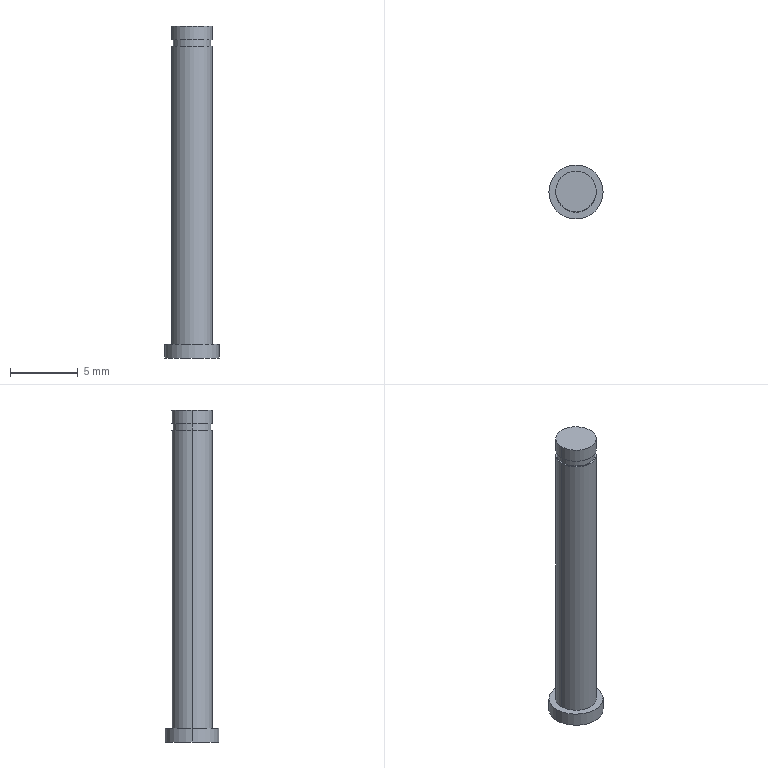Part | STEP file | PN_0099 pin shaft | 1 solid | 13 faces | box 4 x 4 x 24.5 mm | volume 178.223 mm3 | cylinder 8 | plane 5 | commonest cylinder face diameters 3 x4 2.8 x2 4 x2
STEP:
#1=CARTESIAN_POINT('',(0.,0.,0.));
#2=DIRECTION('',(0.,0.,1.));
#3=DIRECTION('',(1.,0.,0.));
#4=AXIS2_PLACEMENT_3D('',#1,#2,#3);
#5=CARTESIAN_POINT('',(1.5,0.,23.5));
#6=VERTEX_POINT('',#5);
#7=CARTESIAN_POINT('',(-1.5,0.,23.5));
#8=VERTEX_POINT('',#7);
#9=CARTESIAN_POINT('',(0.,0.,23.5));
#10=DIRECTION('',(0.,0.,1.));
#11=DIRECTION('',(1.,0.,0.));
#12=AXIS2_PLACEMENT_3D('',#9,#10,#11);
#13=CIRCLE('',#12,1.5);
#14=CARTESIAN_POINT('',(0.,0.,23.5));
#15=DIRECTION('',(0.,0.,-1.));
#16=DIRECTION('',(-1.,0.,0.));
#17=AXIS2_PLACEMENT_3D('',#14,#15,#16);
#18=CYLINDRICAL_SURFACE('',#17,1.5);
#19=CARTESIAN_POINT('',(3.142,0.));
#20=DIRECTION('',(-1.,0.));
#21=VECTOR('',#20,1.);
#22=LINE('',#19,#21);
#23=(GEOMETRIC_REPRESENTATION_CONTEXT(2)PARAMETRIC_REPRESENTATION_CONTEXT()REPRESENTATION_CONTEXT('',''));
#24=DEFINITIONAL_REPRESENTATION('',(#22),#23);
#25=PCURVE('',#18,#24);
#26=CARTESIAN_POINT('',(0.,0.,23.5));
#27=DIRECTION('',(0.,0.,1.));
#28=DIRECTION('',(1.,0.,0.));
#29=AXIS2_PLACEMENT_3D('',#26,#27,#28);
#30=PLANE('',#29);
#31=CARTESIAN_POINT('',(0.,0.));
#32=DIRECTION('',(1.,0.));
#33=AXIS2_PLACEMENT_2D('',#31,#32);
#34=CIRCLE('',#33,1.5);
#35=(GEOMETRIC_REPRESENTATION_CONTEXT(2)PARAMETRIC_REPRESENTATION_CONTEXT()REPRESENTATION_CONTEXT('',''));
#36=DEFINITIONAL_REPRESENTATION('',(#34),#35);
#37=PCURVE('',#30,#36);
#38=SURFACE_CURVE('',#13,(#25,#37),.PCURVE_S1.);
#39=EDGE_CURVE('',#6,#8,#38,.T.);
#40=ORIENTED_EDGE('',*,*,#39,.F.);
#41=CARTESIAN_POINT('',(1.5,0.,22.5));
#42=VERTEX_POINT('',#41);
#43=CARTESIAN_POINT('',(1.5,0.,23.5));
#44=DIRECTION('',(0.,0.,-1.));
#45=VECTOR('',#44,1.);
#46=LINE('',#43,#45);
#47=CARTESIAN_POINT('',(3.142,0.));
#48=DIRECTION('',(0.,1.));
#49=VECTOR('',#48,1.);
#50=LINE('',#47,#49);
#51=(GEOMETRIC_REPRESENTATION_CONTEXT(2)PARAMETRIC_REPRESENTATION_CONTEXT()REPRESENTATION_CONTEXT('',''));
#52=DEFINITIONAL_REPRESENTATION('',(#50),#51);
#53=PCURVE('',#18,#52);
#54=CARTESIAN_POINT('',(0.,0.,23.5));
#55=DIRECTION('',(0.,0.,-1.));
#56=DIRECTION('',(-1.,0.,0.));
#57=AXIS2_PLACEMENT_3D('',#54,#55,#56);
#58=CYLINDRICAL_SURFACE('',#57,1.5);
#59=CARTESIAN_POINT('',(3.142,0.));
#60=DIRECTION('',(0.,1.));
#61=VECTOR('',#60,1.);
#62=LINE('',#59,#61);
#63=(GEOMETRIC_REPRESENTATION_CONTEXT(2)PARAMETRIC_REPRESENTATION_CONTEXT()REPRESENTATION_CONTEXT('',''));
#64=DEFINITIONAL_REPRESENTATION('',(#62),#63);
#65=PCURVE('',#58,#64);
#66=SURFACE_CURVE('',#46,(#53,#65),.PCURVE_S1.);
#67=EDGE_CURVE('',#6,#42,#66,.T.);
#68=ORIENTED_EDGE('',*,*,#67,.T.);
#69=CARTESIAN_POINT('',(-1.5,0.,22.5));
#70=VERTEX_POINT('',#69);
#71=CARTESIAN_POINT('',(0.,0.,22.5));
#72=DIRECTION('',(0.,0.,1.));
#73=DIRECTION('',(1.,0.,0.));
#74=AXIS2_PLACEMENT_3D('',#71,#72,#73);
#75=CIRCLE('',#74,1.5);
#76=CARTESIAN_POINT('',(3.142,1.));
#77=DIRECTION('',(-1.,0.));
#78=VECTOR('',#77,1.);
#79=LINE('',#76,#78);
#80=(GEOMETRIC_REPRESENTATION_CONTEXT(2)PARAMETRIC_REPRESENTATION_CONTEXT()REPRESENTATION_CONTEXT('',''));
#81=DEFINITIONAL_REPRESENTATION('',(#79),#80);
#82=PCURVE('',#18,#81);
#83=CARTESIAN_POINT('',(0.,0.,22.5));
#84=DIRECTION('',(0.,0.,1.));
#85=DIRECTION('',(1.,0.,0.));
#86=AXIS2_PLACEMENT_3D('',#83,#84,#85);
#87=PLANE('',#86);
#88=CARTESIAN_POINT('',(0.,0.));
#89=DIRECTION('',(1.,0.));
#90=AXIS2_PLACEMENT_2D('',#88,#89);
#91=CIRCLE('',#90,1.5);
#92=(GEOMETRIC_REPRESENTATION_CONTEXT(2)PARAMETRIC_REPRESENTATION_CONTEXT()REPRESENTATION_CONTEXT('',''));
#93=DEFINITIONAL_REPRESENTATION('',(#91),#92);
#94=PCURVE('',#87,#93);
#95=SURFACE_CURVE('',#75,(#82,#94),.PCURVE_S1.);
#96=EDGE_CURVE('',#42,#70,#95,.T.);
#97=ORIENTED_EDGE('',*,*,#96,.T.);
#98=CARTESIAN_POINT('',(-1.5,0.,23.5));
#99=DIRECTION('',(0.,0.,-1.));
#100=VECTOR('',#99,1.);
#101=LINE('',#98,#100);
#102=CARTESIAN_POINT('',(0.,0.));
#103=DIRECTION('',(0.,1.));
#104=VECTOR('',#103,1.);
#105=LINE('',#102,#104);
#106=(GEOMETRIC_REPRESENTATION_CONTEXT(2)PARAMETRIC_REPRESENTATION_CONTEXT()REPRESENTATION_CONTEXT('',''));
#107=DEFINITIONAL_REPRESENTATION('',(#105),#106);
#108=PCURVE('',#18,#107);
#109=CARTESIAN_POINT('',(6.283,0.));
#110=DIRECTION('',(0.,1.));
#111=VECTOR('',#110,1.);
#112=LINE('',#109,#111);
#113=(GEOMETRIC_REPRESENTATION_CONTEXT(2)PARAMETRIC_REPRESENTATION_CONTEXT()REPRESENTATION_CONTEXT('',''));
#114=DEFINITIONAL_REPRESENTATION('',(#112),#113);
#115=PCURVE('',#58,#114);
#116=SURFACE_CURVE('',#101,(#108,#115),.PCURVE_S1.);
#117=EDGE_CURVE('',#8,#70,#116,.T.);
#118=ORIENTED_EDGE('',*,*,#117,.F.);
#119=EDGE_LOOP('',(#40,#68,#97,#118));
#120=FACE_BOUND('',#119,.T.);
#121=ADVANCED_FACE('',(#120),#18,.T.);
#122=CARTESIAN_POINT('',(1.4,0.,22.5));
#123=VERTEX_POINT('',#122);
#124=CARTESIAN_POINT('',(-1.4,0.,22.5));
#125=VERTEX_POINT('',#124);
#126=CARTESIAN_POINT('',(0.,0.,22.5));
#127=DIRECTION('',(0.,0.,1.));
#128=DIRECTION('',(1.,0.,0.));
#129=AXIS2_PLACEMENT_3D('',#126,#127,#128);
#130=CIRCLE('',#129,1.4);
#131=CARTESIAN_POINT('',(0.,0.,22.5));
#132=DIRECTION('',(0.,0.,-1.));
#133=DIRECTION('',(-1.,0.,0.));
#134=AXIS2_PLACEMENT_3D('',#131,#132,#133);
#135=CYLINDRICAL_SURFACE('',#134,1.4);
#136=CARTESIAN_POINT('',(3.142,0.));
#137=DIRECTION('',(-1.,0.));
#138=VECTOR('',#137,1.);
#139=LINE('',#136,#138);
#140=(GEOMETRIC_REPRESENTATION_CONTEXT(2)PARAMETRIC_REPRESENTATION_CONTEXT()REPRESENTATION_CONTEXT('',''));
#141=DEFINITIONAL_REPRESENTATION('',(#139),#140);
#142=PCURVE('',#135,#141);
#143=CARTESIAN_POINT('',(0.,0.));
#144=DIRECTION('',(1.,0.));
#145=AXIS2_PLACEMENT_2D('',#143,#144);
#146=CIRCLE('',#145,1.4);
#147=(GEOMETRIC_REPRESENTATION_CONTEXT(2)PARAMETRIC_REPRESENTATION_CONTEXT()REPRESENTATION_CONTEXT('',''));
#148=DEFINITIONAL_REPRESENTATION('',(#146),#147);
#149=PCURVE('',#87,#148);
#150=SURFACE_CURVE('',#130,(#142,#149),.PCURVE_S1.);
#151=EDGE_CURVE('',#123,#125,#150,.T.);
#152=ORIENTED_EDGE('',*,*,#151,.F.);
#153=CARTESIAN_POINT('',(1.4,0.,22.));
#154=VERTEX_POINT('',#153);
#155=CARTESIAN_POINT('',(1.4,0.,22.5));
#156=DIRECTION('',(0.,0.,-1.));
#157=VECTOR('',#156,1.);
#158=LINE('',#155,#157);
#159=CARTESIAN_POINT('',(3.142,0.));
#160=DIRECTION('',(0.,1.));
#161=VECTOR('',#160,1.);
#162=LINE('',#159,#161);
#163=(GEOMETRIC_REPRESENTATION_CONTEXT(2)PARAMETRIC_REPRESENTATION_CONTEXT()REPRESENTATION_CONTEXT('',''));
#164=DEFINITIONAL_REPRESENTATION('',(#162),#163);
#165=PCURVE('',#135,#164);
#166=CARTESIAN_POINT('',(0.,0.,22.5));
#167=DIRECTION('',(0.,0.,-1.));
#168=DIRECTION('',(-1.,0.,0.));
#169=AXIS2_PLACEMENT_3D('',#166,#167,#168);
#170=CYLINDRICAL_SURFACE('',#169,1.4);
#171=CARTESIAN_POINT('',(3.142,0.));
#172=DIRECTION('',(0.,1.));
#173=VECTOR('',#172,1.);
#174=LINE('',#171,#173);
#175=(GEOMETRIC_REPRESENTATION_CONTEXT(2)PARAMETRIC_REPRESENTATION_CONTEXT()REPRESENTATION_CONTEXT('',''));
#176=DEFINITIONAL_REPRESENTATION('',(#174),#175);
#177=PCURVE('',#170,#176);
#178=SURFACE_CURVE('',#158,(#165,#177),.PCURVE_S1.);
#179=EDGE_CURVE('',#123,#154,#178,.T.);
#180=ORIENTED_EDGE('',*,*,#179,.T.);
#181=CARTESIAN_POINT('',(-1.4,0.,22.));
#182=VERTEX_POINT('',#181);
#183=CARTESIAN_POINT('',(0.,0.,22.));
#184=DIRECTION('',(0.,0.,1.));
#185=DIRECTION('',(1.,0.,0.));
#186=AXIS2_PLACEMENT_3D('',#183,#184,#185);
#187=CIRCLE('',#186,1.4);
#188=CARTESIAN_POINT('',(3.142,0.5));
#189=DIRECTION('',(-1.,0.));
#190=VECTOR('',#189,1.);
#191=LINE('',#188,#190);
#192=(GEOMETRIC_REPRESENTATION_CONTEXT(2)PARAMETRIC_REPRESENTATION_CONTEXT()REPRESENTATION_CONTEXT('',''));
#193=DEFINITIONAL_REPRESENTATION('',(#191),#192);
#194=PCURVE('',#135,#193);
#195=CARTESIAN_POINT('',(0.,0.,22.));
#196=DIRECTION('',(0.,0.,1.));
#197=DIRECTION('',(1.,0.,0.));
#198=AXIS2_PLACEMENT_3D('',#195,#196,#197);
#199=PLANE('',#198);
#200=CARTESIAN_POINT('',(0.,0.));
#201=DIRECTION('',(1.,0.));
#202=AXIS2_PLACEMENT_2D('',#200,#201);
#203=CIRCLE('',#202,1.4);
#204=(GEOMETRIC_REPRESENTATION_CONTEXT(2)PARAMETRIC_REPRESENTATION_CONTEXT()REPRESENTATION_CONTEXT('',''));
#205=DEFINITIONAL_REPRESENTATION('',(#203),#204);
#206=PCURVE('',#199,#205);
#207=SURFACE_CURVE('',#187,(#194,#206),.PCURVE_S1.);
#208=EDGE_CURVE('',#154,#182,#207,.T.);
#209=ORIENTED_EDGE('',*,*,#208,.T.);
#210=CARTESIAN_POINT('',(-1.4,0.,22.5));
#211=DIRECTION('',(0.,0.,-1.));
#212=VECTOR('',#211,1.);
#213=LINE('',#210,#212);
#214=CARTESIAN_POINT('',(0.,0.));
#215=DIRECTION('',(0.,1.));
#216=VECTOR('',#215,1.);
#217=LINE('',#214,#216);
#218=(GEOMETRIC_REPRESENTATION_CONTEXT(2)PARAMETRIC_REPRESENTATION_CONTEXT()REPRESENTATION_CONTEXT('',''));
#219=DEFINITIONAL_REPRESENTATION('',(#217),#218);
#220=PCURVE('',#135,#219);
#221=CARTESIAN_POINT('',(6.283,0.));
#222=DIRECTION('',(0.,1.));
#223=VECTOR('',#222,1.);
#224=LINE('',#221,#223);
#225=(GEOMETRIC_REPRESENTATION_CONTEXT(2)PARAMETRIC_REPRESENTATION_CONTEXT()REPRESENTATION_CONTEXT('',''));
#226=DEFINITIONAL_REPRESENTATION('',(#224),#225);
#227=PCURVE('',#170,#226);
#228=SURFACE_CURVE('',#213,(#220,#227),.PCURVE_S1.);
#229=EDGE_CURVE('',#125,#182,#228,.T.);
#230=ORIENTED_EDGE('',*,*,#229,.F.);
#231=EDGE_LOOP('',(#152,#180,#209,#230));
#232=FACE_BOUND('',#231,.T.);
#233=ADVANCED_FACE('',(#232),#135,.T.);
#234=CARTESIAN_POINT('',(-2.,0.,-1.));
#235=VERTEX_POINT('',#234);
#236=CARTESIAN_POINT('',(2.,0.,-1.));
#237=VERTEX_POINT('',#236);
#238=CARTESIAN_POINT('',(0.,0.,-1.));
#239=DIRECTION('',(0.,0.,-1.));
#240=DIRECTION('',(-1.,0.,0.));
#241=AXIS2_PLACEMENT_3D('',#238,#239,#240);
#242=CIRCLE('',#241,2.);
#243=CARTESIAN_POINT('',(0.,0.,-1.));
#244=DIRECTION('',(0.,0.,1.));
#245=DIRECTION('',(1.,0.,0.));
#246=AXIS2_PLACEMENT_3D('',#243,#244,#245);
#247=CYLINDRICAL_SURFACE('',#246,2.);
#248=CARTESIAN_POINT('',(3.142,0.));
#249=DIRECTION('',(-1.,0.));
#250=VECTOR('',#249,1.);
#251=LINE('',#248,#250);
#252=(GEOMETRIC_REPRESENTATION_CONTEXT(2)PARAMETRIC_REPRESENTATION_CONTEXT()REPRESENTATION_CONTEXT('',''));
#253=DEFINITIONAL_REPRESENTATION('',(#251),#252);
#254=PCURVE('',#247,#253);
#255=CARTESIAN_POINT('',(0.,0.,-1.));
#256=DIRECTION('',(0.,0.,-1.));
#257=DIRECTION('',(-1.,0.,0.));
#258=AXIS2_PLACEMENT_3D('',#255,#256,#257);
#259=PLANE('',#258);
#260=CARTESIAN_POINT('',(0.,0.));
#261=DIRECTION('',(1.,0.));
#262=AXIS2_PLACEMENT_2D('',#260,#261);
#263=CIRCLE('',#262,2.);
#264=(GEOMETRIC_REPRESENTATION_CONTEXT(2)PARAMETRIC_REPRESENTATION_CONTEXT()REPRESENTATION_CONTEXT('',''));
#265=DEFINITIONAL_REPRESENTATION('',(#263),#264);
#266=PCURVE('',#259,#265);
#267=SURFACE_CURVE('',#242,(#254,#266),.PCURVE_S1.);
#268=EDGE_CURVE('',#235,#237,#267,.T.);
#269=ORIENTED_EDGE('',*,*,#268,.F.);
#270=CARTESIAN_POINT('',(-2.,0.,0.));
#271=VERTEX_POINT('',#270);
#272=CARTESIAN_POINT('',(-2.,0.,-1.));
#273=DIRECTION('',(0.,0.,1.));
#274=VECTOR('',#273,1.);
#275=LINE('',#272,#274);
#276=CARTESIAN_POINT('',(3.142,0.));
#277=DIRECTION('',(0.,1.));
#278=VECTOR('',#277,1.);
#279=LINE('',#276,#278);
#280=(GEOMETRIC_REPRESENTATION_CONTEXT(2)PARAMETRIC_REPRESENTATION_CONTEXT()REPRESENTATION_CONTEXT('',''));
#281=DEFINITIONAL_REPRESENTATION('',(#279),#280);
#282=PCURVE('',#247,#281);
#283=CARTESIAN_POINT('',(0.,0.,-1.));
#284=DIRECTION('',(0.,0.,1.));
#285=DIRECTION('',(1.,0.,0.));
#286=AXIS2_PLACEMENT_3D('',#283,#284,#285);
#287=CYLINDRICAL_SURFACE('',#286,2.);
#288=CARTESIAN_POINT('',(3.142,0.));
#289=DIRECTION('',(0.,1.));
#290=VECTOR('',#289,1.);
#291=LINE('',#288,#290);
#292=(GEOMETRIC_REPRESENTATION_CONTEXT(2)PARAMETRIC_REPRESENTATION_CONTEXT()REPRESENTATION_CONTEXT('',''));
#293=DEFINITIONAL_REPRESENTATION('',(#291),#292);
#294=PCURVE('',#287,#293);
#295=SURFACE_CURVE('',#275,(#282,#294),.PCURVE_S1.);
#296=EDGE_CURVE('',#235,#271,#295,.T.);
#297=ORIENTED_EDGE('',*,*,#296,.T.);
#298=CARTESIAN_POINT('',(2.,0.,0.));
#299=VERTEX_POINT('',#298);
#300=CARTESIAN_POINT('',(0.,0.,0.));
#301=DIRECTION('',(0.,0.,-1.));
#302=DIRECTION('',(-1.,0.,0.));
#303=AXIS2_PLACEMENT_3D('',#300,#301,#302);
#304=CIRCLE('',#303,2.);
#305=CARTESIAN_POINT('',(3.142,1.));
#306=DIRECTION('',(-1.,0.));
#307=VECTOR('',#306,1.);
#308=LINE('',#305,#307);
#309=(GEOMETRIC_REPRESENTATION_CONTEXT(2)PARAMETRIC_REPRESENTATION_CONTEXT()REPRESENTATION_CONTEXT('',''));
#310=DEFINITIONAL_REPRESENTATION('',(#308),#309);
#311=PCURVE('',#247,#310);
#312=CARTESIAN_POINT('',(0.,0.,0.));
#313=DIRECTION('',(0.,0.,-1.));
#314=DIRECTION('',(-1.,0.,0.));
#315=AXIS2_PLACEMENT_3D('',#312,#313,#314);
#316=PLANE('',#315);
#317=CARTESIAN_POINT('',(0.,0.));
#318=DIRECTION('',(1.,0.));
#319=AXIS2_PLACEMENT_2D('',#317,#318);
#320=CIRCLE('',#319,2.);
#321=(GEOMETRIC_REPRESENTATION_CONTEXT(2)PARAMETRIC_REPRESENTATION_CONTEXT()REPRESENTATION_CONTEXT('',''));
#322=DEFINITIONAL_REPRESENTATION('',(#320),#321);
#323=PCURVE('',#316,#322);
#324=SURFACE_CURVE('',#304,(#311,#323),.PCURVE_S1.);
#325=EDGE_CURVE('',#271,#299,#324,.T.);
#326=ORIENTED_EDGE('',*,*,#325,.T.);
#327=CARTESIAN_POINT('',(2.,0.,-1.));
#328=DIRECTION('',(0.,0.,1.));
#329=VECTOR('',#328,1.);
#330=LINE('',#327,#329);
#331=CARTESIAN_POINT('',(0.,0.));
#332=DIRECTION('',(0.,1.));
#333=VECTOR('',#332,1.);
#334=LINE('',#331,#333);
#335=(GEOMETRIC_REPRESENTATION_CONTEXT(2)PARAMETRIC_REPRESENTATION_CONTEXT()REPRESENTATION_CONTEXT('',''));
#336=DEFINITIONAL_REPRESENTATION('',(#334),#335);
#337=PCURVE('',#247,#336);
#338=CARTESIAN_POINT('',(6.283,0.));
#339=DIRECTION('',(0.,1.));
#340=VECTOR('',#339,1.);
#341=LINE('',#338,#340);
#342=(GEOMETRIC_REPRESENTATION_CONTEXT(2)PARAMETRIC_REPRESENTATION_CONTEXT()REPRESENTATION_CONTEXT('',''));
#343=DEFINITIONAL_REPRESENTATION('',(#341),#342);
#344=PCURVE('',#287,#343);
#345=SURFACE_CURVE('',#330,(#337,#344),.PCURVE_S1.);
#346=EDGE_CURVE('',#237,#299,#345,.T.);
#347=ORIENTED_EDGE('',*,*,#346,.F.);
#348=EDGE_LOOP('',(#269,#297,#326,#347));
#349=FACE_BOUND('',#348,.T.);
#350=ADVANCED_FACE('',(#349),#247,.T.);
#351=CARTESIAN_POINT('',(1.5,0.,22.));
#352=VERTEX_POINT('',#351);
#353=CARTESIAN_POINT('',(-1.5,0.,22.));
#354=VERTEX_POINT('',#353);
#355=CARTESIAN_POINT('',(0.,0.,22.));
#356=DIRECTION('',(0.,0.,1.));
#357=DIRECTION('',(1.,0.,0.));
#358=AXIS2_PLACEMENT_3D('',#355,#356,#357);
#359=CIRCLE('',#358,1.5);
#360=CARTESIAN_POINT('',(0.,0.,22.));
#361=DIRECTION('',(0.,0.,-1.));
#362=DIRECTION('',(-1.,0.,0.));
#363=AXIS2_PLACEMENT_3D('',#360,#361,#362);
#364=CYLINDRICAL_SURFACE('',#363,1.5);
#365=CARTESIAN_POINT('',(3.142,0.));
#366=DIRECTION('',(-1.,0.));
#367=VECTOR('',#366,1.);
#368=LINE('',#365,#367);
#369=(GEOMETRIC_REPRESENTATION_CONTEXT(2)PARAMETRIC_REPRESENTATION_CONTEXT()REPRESENTATION_CONTEXT('',''));
#370=DEFINITIONAL_REPRESENTATION('',(#368),#369);
#371=PCURVE('',#364,#370);
#372=CARTESIAN_POINT('',(0.,0.));
#373=DIRECTION('',(1.,0.));
#374=AXIS2_PLACEMENT_2D('',#372,#373);
#375=CIRCLE('',#374,1.5);
#376=(GEOMETRIC_REPRESENTATION_CONTEXT(2)PARAMETRIC_REPRESENTATION_CONTEXT()REPRESENTATION_CONTEXT('',''));
#377=DEFINITIONAL_REPRESENTATION('',(#375),#376);
#378=PCURVE('',#199,#377);
#379=SURFACE_CURVE('',#359,(#371,#378),.PCURVE_S1.);
#380=EDGE_CURVE('',#352,#354,#379,.T.);
#381=ORIENTED_EDGE('',*,*,#380,.F.);
#382=CARTESIAN_POINT('',(1.5,0.,0.));
#383=VERTEX_POINT('',#382);
#384=CARTESIAN_POINT('',(1.5,0.,22.));
#385=DIRECTION('',(0.,0.,-1.));
#386=VECTOR('',#385,1.);
#387=LINE('',#384,#386);
#388=CARTESIAN_POINT('',(3.142,0.));
#389=DIRECTION('',(0.,1.));
#390=VECTOR('',#389,1.);
#391=LINE('',#388,#390);
#392=(GEOMETRIC_REPRESENTATION_CONTEXT(2)PARAMETRIC_REPRESENTATION_CONTEXT()REPRESENTATION_CONTEXT('',''));
#393=DEFINITIONAL_REPRESENTATION('',(#391),#392);
#394=PCURVE('',#364,#393);
#395=CARTESIAN_POINT('',(0.,0.,22.));
#396=DIRECTION('',(0.,0.,-1.));
#397=DIRECTION('',(-1.,0.,0.));
#398=AXIS2_PLACEMENT_3D('',#395,#396,#397);
#399=CYLINDRICAL_SURFACE('',#398,1.5);
#400=CARTESIAN_POINT('',(3.142,0.));
#401=DIRECTION('',(0.,1.));
#402=VECTOR('',#401,1.);
#403=LINE('',#400,#402);
#404=(GEOMETRIC_REPRESENTATION_CONTEXT(2)PARAMETRIC_REPRESENTATION_CONTEXT()REPRESENTATION_CONTEXT('',''));
#405=DEFINITIONAL_REPRESENTATION('',(#403),#404);
#406=PCURVE('',#399,#405);
#407=SURFACE_CURVE('',#387,(#394,#406),.PCURVE_S1.);
#408=EDGE_CURVE('',#352,#383,#407,.T.);
#409=ORIENTED_EDGE('',*,*,#408,.T.);
#410=CARTESIAN_POINT('',(-1.5,0.,0.));
#411=VERTEX_POINT('',#410);
#412=CARTESIAN_POINT('',(0.,0.,0.));
#413=DIRECTION('',(0.,0.,-1.));
#414=DIRECTION('',(-1.,0.,0.));
#415=AXIS2_PLACEMENT_3D('',#412,#413,#414);
#416=CIRCLE('',#415,1.5);
#417=CARTESIAN_POINT('',(0.,22.));
#418=DIRECTION('',(1.,0.));
#419=VECTOR('',#418,1.);
#420=LINE('',#417,#419);
#421=(GEOMETRIC_REPRESENTATION_CONTEXT(2)PARAMETRIC_REPRESENTATION_CONTEXT()REPRESENTATION_CONTEXT('',''));
#422=DEFINITIONAL_REPRESENTATION('',(#420),#421);
#423=PCURVE('',#364,#422);
#424=CARTESIAN_POINT('',(0.,0.));
#425=DIRECTION('',(1.,0.));
#426=AXIS2_PLACEMENT_2D('',#424,#425);
#427=CIRCLE('',#426,1.5);
#428=(GEOMETRIC_REPRESENTATION_CONTEXT(2)PARAMETRIC_REPRESENTATION_CONTEXT()REPRESENTATION_CONTEXT('',''));
#429=DEFINITIONAL_REPRESENTATION('',(#427),#428);
#430=PCURVE('',#316,#429);
#431=SURFACE_CURVE('',#416,(#423,#430),.PCURVE_S1.);
#432=EDGE_CURVE('',#411,#383,#431,.T.);
#433=ORIENTED_EDGE('',*,*,#432,.F.);
#434=CARTESIAN_POINT('',(-1.5,0.,22.));
#435=DIRECTION('',(0.,0.,-1.));
#436=VECTOR('',#435,1.);
#437=LINE('',#434,#436);
#438=CARTESIAN_POINT('',(0.,0.));
#439=DIRECTION('',(0.,1.));
#440=VECTOR('',#439,1.);
#441=LINE('',#438,#440);
#442=(GEOMETRIC_REPRESENTATION_CONTEXT(2)PARAMETRIC_REPRESENTATION_CONTEXT()REPRESENTATION_CONTEXT('',''));
#443=DEFINITIONAL_REPRESENTATION('',(#441),#442);
#444=PCURVE('',#364,#443);
#445=CARTESIAN_POINT('',(6.283,0.));
#446=DIRECTION('',(0.,1.));
#447=VECTOR('',#446,1.);
#448=LINE('',#445,#447);
#449=(GEOMETRIC_REPRESENTATION_CONTEXT(2)PARAMETRIC_REPRESENTATION_CONTEXT()REPRESENTATION_CONTEXT('',''));
#450=DEFINITIONAL_REPRESENTATION('',(#448),#449);
#451=PCURVE('',#399,#450);
#452=SURFACE_CURVE('',#437,(#444,#451),.PCURVE_S1.);
#453=EDGE_CURVE('',#354,#411,#452,.T.);
#454=ORIENTED_EDGE('',*,*,#453,.F.);
#455=EDGE_LOOP('',(#381,#409,#433,#454));
#456=FACE_BOUND('',#455,.T.);
#457=ADVANCED_FACE('',(#456),#364,.T.);
#458=CARTESIAN_POINT('',(0.,0.,22.));
#459=DIRECTION('',(0.,0.,1.));
#460=DIRECTION('',(1.,0.,0.));
#461=AXIS2_PLACEMENT_3D('',#458,#459,#460);
#462=CIRCLE('',#461,1.5);
#463=CARTESIAN_POINT('',(0.,0.));
#464=DIRECTION('',(1.,0.));
#465=AXIS2_PLACEMENT_2D('',#463,#464);
#466=CIRCLE('',#465,1.5);
#467=(GEOMETRIC_REPRESENTATION_CONTEXT(2)PARAMETRIC_REPRESENTATION_CONTEXT()REPRESENTATION_CONTEXT('',''));
#468=DEFINITIONAL_REPRESENTATION('',(#466),#467);
#469=PCURVE('',#199,#468);
#470=CARTESIAN_POINT('',(9.425,0.));
#471=DIRECTION('',(-1.,0.));
#472=VECTOR('',#471,1.);
#473=LINE('',#470,#472);
#474=(GEOMETRIC_REPRESENTATION_CONTEXT(2)PARAMETRIC_REPRESENTATION_CONTEXT()REPRESENTATION_CONTEXT('',''));
#475=DEFINITIONAL_REPRESENTATION('',(#473),#474);
#476=PCURVE('',#399,#475);
#477=SURFACE_CURVE('',#462,(#469,#476),.PCURVE_S1.);
#478=EDGE_CURVE('',#354,#352,#477,.T.);
#479=ORIENTED_EDGE('',*,*,#478,.T.);
#480=ORIENTED_EDGE('',*,*,#380,.T.);
#481=EDGE_LOOP('',(#479,#480));
#482=FACE_BOUND('',#481,.T.);
#483=CARTESIAN_POINT('',(0.,0.,22.));
#484=DIRECTION('',(0.,0.,1.));
#485=DIRECTION('',(1.,0.,0.));
#486=AXIS2_PLACEMENT_3D('',#483,#484,#485);
#487=CIRCLE('',#486,1.4);
#488=CARTESIAN_POINT('',(0.,0.));
#489=DIRECTION('',(1.,0.));
#490=AXIS2_PLACEMENT_2D('',#488,#489);
#491=CIRCLE('',#490,1.4);
#492=(GEOMETRIC_REPRESENTATION_CONTEXT(2)PARAMETRIC_REPRESENTATION_CONTEXT()REPRESENTATION_CONTEXT('',''));
#493=DEFINITIONAL_REPRESENTATION('',(#491),#492);
#494=PCURVE('',#199,#493);
#495=CARTESIAN_POINT('',(9.425,0.5));
#496=DIRECTION('',(-1.,0.));
#497=VECTOR('',#496,1.);
#498=LINE('',#495,#497);
#499=(GEOMETRIC_REPRESENTATION_CONTEXT(2)PARAMETRIC_REPRESENTATION_CONTEXT()REPRESENTATION_CONTEXT('',''));
#500=DEFINITIONAL_REPRESENTATION('',(#498),#499);
#501=PCURVE('',#170,#500);
#502=SURFACE_CURVE('',#487,(#494,#501),.PCURVE_S1.);
#503=EDGE_CURVE('',#182,#154,#502,.T.);
#504=ORIENTED_EDGE('',*,*,#503,.F.);
#505=ORIENTED_EDGE('',*,*,#208,.F.);
#506=EDGE_LOOP('',(#504,#505));
#507=FACE_BOUND('',#506,.T.);
#508=ADVANCED_FACE('',(#482,#507),#199,.T.);
#509=ORIENTED_EDGE('',*,*,#408,.F.);
#510=ORIENTED_EDGE('',*,*,#478,.F.);
#511=ORIENTED_EDGE('',*,*,#453,.T.);
#512=CARTESIAN_POINT('',(0.,0.,0.));
#513=DIRECTION('',(0.,0.,-1.));
#514=DIRECTION('',(-1.,0.,0.));
#515=AXIS2_PLACEMENT_3D('',#512,#513,#514);
#516=CIRCLE('',#515,1.5);
#517=CARTESIAN_POINT('',(0.,22.));
#518=DIRECTION('',(1.,0.));
#519=VECTOR('',#518,1.);
#520=LINE('',#517,#519);
#521=(GEOMETRIC_REPRESENTATION_CONTEXT(2)PARAMETRIC_REPRESENTATION_CONTEXT()REPRESENTATION_CONTEXT('',''));
#522=DEFINITIONAL_REPRESENTATION('',(#520),#521);
#523=PCURVE('',#399,#522);
#524=CARTESIAN_POINT('',(0.,0.));
#525=DIRECTION('',(1.,0.));
#526=AXIS2_PLACEMENT_2D('',#524,#525);
#527=CIRCLE('',#526,1.5);
#528=(GEOMETRIC_REPRESENTATION_CONTEXT(2)PARAMETRIC_REPRESENTATION_CONTEXT()REPRESENTATION_CONTEXT('',''));
#529=DEFINITIONAL_REPRESENTATION('',(#527),#528);
#530=PCURVE('',#316,#529);
#531=SURFACE_CURVE('',#516,(#523,#530),.PCURVE_S1.);
#532=EDGE_CURVE('',#383,#411,#531,.T.);
#533=ORIENTED_EDGE('',*,*,#532,.F.);
#534=EDGE_LOOP('',(#509,#510,#511,#533));
#535=FACE_BOUND('',#534,.T.);
#536=ADVANCED_FACE('',(#535),#399,.T.);
#537=CARTESIAN_POINT('',(0.,0.,0.));
#538=DIRECTION('',(0.,0.,-1.));
#539=DIRECTION('',(-1.,0.,0.));
#540=AXIS2_PLACEMENT_3D('',#537,#538,#539);
#541=CIRCLE('',#540,2.);
#542=CARTESIAN_POINT('',(0.,0.));
#543=DIRECTION('',(1.,0.));
#544=AXIS2_PLACEMENT_2D('',#542,#543);
#545=CIRCLE('',#544,2.);
#546=(GEOMETRIC_REPRESENTATION_CONTEXT(2)PARAMETRIC_REPRESENTATION_CONTEXT()REPRESENTATION_CONTEXT('',''));
#547=DEFINITIONAL_REPRESENTATION('',(#545),#546);
#548=PCURVE('',#316,#547);
#549=CARTESIAN_POINT('',(9.425,1.));
#550=DIRECTION('',(-1.,0.));
#551=VECTOR('',#550,1.);
#552=LINE('',#549,#551);
#553=(GEOMETRIC_REPRESENTATION_CONTEXT(2)PARAMETRIC_REPRESENTATION_CONTEXT()REPRESENTATION_CONTEXT('',''));
#554=DEFINITIONAL_REPRESENTATION('',(#552),#553);
#555=PCURVE('',#287,#554);
#556=SURFACE_CURVE('',#541,(#548,#555),.PCURVE_S1.);
#557=EDGE_CURVE('',#299,#271,#556,.T.);
#558=ORIENTED_EDGE('',*,*,#557,.F.);
#559=ORIENTED_EDGE('',*,*,#325,.F.);
#560=EDGE_LOOP('',(#558,#559));
#561=FACE_BOUND('',#560,.T.);
#562=ORIENTED_EDGE('',*,*,#432,.T.);
#563=ORIENTED_EDGE('',*,*,#532,.T.);
#564=EDGE_LOOP('',(#562,#563));
#565=FACE_BOUND('',#564,.T.);
#566=ADVANCED_FACE('',(#561,#565),#316,.F.);
#567=ORIENTED_EDGE('',*,*,#296,.F.);
#568=CARTESIAN_POINT('',(0.,0.,-1.));
#569=DIRECTION('',(0.,0.,-1.));
#570=DIRECTION('',(-1.,0.,0.));
#571=AXIS2_PLACEMENT_3D('',#568,#569,#570);
#572=CIRCLE('',#571,2.);
#573=CARTESIAN_POINT('',(9.425,0.));
#574=DIRECTION('',(-1.,0.));
#575=VECTOR('',#574,1.);
#576=LINE('',#573,#575);
#577=(GEOMETRIC_REPRESENTATION_CONTEXT(2)PARAMETRIC_REPRESENTATION_CONTEXT()REPRESENTATION_CONTEXT('',''));
#578=DEFINITIONAL_REPRESENTATION('',(#576),#577);
#579=PCURVE('',#287,#578);
#580=CARTESIAN_POINT('',(0.,0.));
#581=DIRECTION('',(1.,0.));
#582=AXIS2_PLACEMENT_2D('',#580,#581);
#583=CIRCLE('',#582,2.);
#584=(GEOMETRIC_REPRESENTATION_CONTEXT(2)PARAMETRIC_REPRESENTATION_CONTEXT()REPRESENTATION_CONTEXT('',''));
#585=DEFINITIONAL_REPRESENTATION('',(#583),#584);
#586=PCURVE('',#259,#585);
#587=SURFACE_CURVE('',#572,(#579,#586),.PCURVE_S1.);
#588=EDGE_CURVE('',#237,#235,#587,.T.);
#589=ORIENTED_EDGE('',*,*,#588,.F.);
#590=ORIENTED_EDGE('',*,*,#346,.T.);
#591=ORIENTED_EDGE('',*,*,#557,.T.);
#592=EDGE_LOOP('',(#567,#589,#590,#591));
#593=FACE_BOUND('',#592,.T.);
#594=ADVANCED_FACE('',(#593),#287,.T.);
#595=ORIENTED_EDGE('',*,*,#588,.T.);
#596=ORIENTED_EDGE('',*,*,#268,.T.);
#597=EDGE_LOOP('',(#595,#596));
#598=FACE_BOUND('',#597,.T.);
#599=ADVANCED_FACE('',(#598),#259,.T.);
#600=ORIENTED_EDGE('',*,*,#179,.F.);
#601=CARTESIAN_POINT('',(0.,0.,22.5));
#602=DIRECTION('',(0.,0.,1.));
#603=DIRECTION('',(1.,0.,0.));
#604=AXIS2_PLACEMENT_3D('',#601,#602,#603);
#605=CIRCLE('',#604,1.4);
#606=CARTESIAN_POINT('',(9.425,0.));
#607=DIRECTION('',(-1.,0.));
#608=VECTOR('',#607,1.);
#609=LINE('',#606,#608);
#610=(GEOMETRIC_REPRESENTATION_CONTEXT(2)PARAMETRIC_REPRESENTATION_CONTEXT()REPRESENTATION_CONTEXT('',''));
#611=DEFINITIONAL_REPRESENTATION('',(#609),#610);
#612=PCURVE('',#170,#611);
#613=CARTESIAN_POINT('',(0.,0.));
#614=DIRECTION('',(1.,0.));
#615=AXIS2_PLACEMENT_2D('',#613,#614);
#616=CIRCLE('',#615,1.4);
#617=(GEOMETRIC_REPRESENTATION_CONTEXT(2)PARAMETRIC_REPRESENTATION_CONTEXT()REPRESENTATION_CONTEXT('',''));
#618=DEFINITIONAL_REPRESENTATION('',(#616),#617);
#619=PCURVE('',#87,#618);
#620=SURFACE_CURVE('',#605,(#612,#619),.PCURVE_S1.);
#621=EDGE_CURVE('',#125,#123,#620,.T.);
#622=ORIENTED_EDGE('',*,*,#621,.F.);
#623=ORIENTED_EDGE('',*,*,#229,.T.);
#624=ORIENTED_EDGE('',*,*,#503,.T.);
#625=EDGE_LOOP('',(#600,#622,#623,#624));
#626=FACE_BOUND('',#625,.T.);
#627=ADVANCED_FACE('',(#626),#170,.T.);
#628=CARTESIAN_POINT('',(0.,0.,22.5));
#629=DIRECTION('',(0.,0.,1.));
#630=DIRECTION('',(1.,0.,0.));
#631=AXIS2_PLACEMENT_3D('',#628,#629,#630);
#632=CIRCLE('',#631,1.5);
#633=CARTESIAN_POINT('',(0.,0.));
#634=DIRECTION('',(1.,0.));
#635=AXIS2_PLACEMENT_2D('',#633,#634);
#636=CIRCLE('',#635,1.5);
#637=(GEOMETRIC_REPRESENTATION_CONTEXT(2)PARAMETRIC_REPRESENTATION_CONTEXT()REPRESENTATION_CONTEXT('',''));
#638=DEFINITIONAL_REPRESENTATION('',(#636),#637);
#639=PCURVE('',#87,#638);
#640=CARTESIAN_POINT('',(9.425,1.));
#641=DIRECTION('',(-1.,0.));
#642=VECTOR('',#641,1.);
#643=LINE('',#640,#642);
#644=(GEOMETRIC_REPRESENTATION_CONTEXT(2)PARAMETRIC_REPRESENTATION_CONTEXT()REPRESENTATION_CONTEXT('',''));
#645=DEFINITIONAL_REPRESENTATION('',(#643),#644);
#646=PCURVE('',#58,#645);
#647=SURFACE_CURVE('',#632,(#639,#646),.PCURVE_S1.);
#648=EDGE_CURVE('',#70,#42,#647,.T.);
#649=ORIENTED_EDGE('',*,*,#648,.F.);
#650=ORIENTED_EDGE('',*,*,#96,.F.);
#651=EDGE_LOOP('',(#649,#650));
#652=FACE_BOUND('',#651,.T.);
#653=ORIENTED_EDGE('',*,*,#621,.T.);
#654=ORIENTED_EDGE('',*,*,#151,.T.);
#655=EDGE_LOOP('',(#653,#654));
#656=FACE_BOUND('',#655,.T.);
#657=ADVANCED_FACE('',(#652,#656),#87,.F.);
#658=ORIENTED_EDGE('',*,*,#67,.F.);
#659=CARTESIAN_POINT('',(0.,0.,23.5));
#660=DIRECTION('',(0.,0.,1.));
#661=DIRECTION('',(1.,0.,0.));
#662=AXIS2_PLACEMENT_3D('',#659,#660,#661);
#663=CIRCLE('',#662,1.5);
#664=CARTESIAN_POINT('',(9.425,0.));
#665=DIRECTION('',(-1.,0.));
#666=VECTOR('',#665,1.);
#667=LINE('',#664,#666);
#668=(GEOMETRIC_REPRESENTATION_CONTEXT(2)PARAMETRIC_REPRESENTATION_CONTEXT()REPRESENTATION_CONTEXT('',''));
#669=DEFINITIONAL_REPRESENTATION('',(#667),#668);
#670=PCURVE('',#58,#669);
#671=CARTESIAN_POINT('',(0.,0.));
#672=DIRECTION('',(1.,0.));
#673=AXIS2_PLACEMENT_2D('',#671,#672);
#674=CIRCLE('',#673,1.5);
#675=(GEOMETRIC_REPRESENTATION_CONTEXT(2)PARAMETRIC_REPRESENTATION_CONTEXT()REPRESENTATION_CONTEXT('',''));
#676=DEFINITIONAL_REPRESENTATION('',(#674),#675);
#677=PCURVE('',#30,#676);
#678=SURFACE_CURVE('',#663,(#670,#677),.PCURVE_S1.);
#679=EDGE_CURVE('',#8,#6,#678,.T.);
#680=ORIENTED_EDGE('',*,*,#679,.F.);
#681=ORIENTED_EDGE('',*,*,#117,.T.);
#682=ORIENTED_EDGE('',*,*,#648,.T.);
#683=EDGE_LOOP('',(#658,#680,#681,#682));
#684=FACE_BOUND('',#683,.T.);
#685=ADVANCED_FACE('',(#684),#58,.T.);
#686=ORIENTED_EDGE('',*,*,#679,.T.);
#687=ORIENTED_EDGE('',*,*,#39,.T.);
#688=EDGE_LOOP('',(#686,#687));
#689=FACE_BOUND('',#688,.T.);
#690=ADVANCED_FACE('',(#689),#30,.T.);
#691=CLOSED_SHELL('',(#121,#233,#350,#457,#508,#536,#566,#594,#599,#627,#657,#685,#690));
#692=MANIFOLD_SOLID_BREP('',#691);
#693=(LENGTH_UNIT()NAMED_UNIT(*)SI_UNIT(.MILLI.,.METRE.));
#694=UNCERTAINTY_MEASURE_WITH_UNIT(LENGTH_MEASURE(0.0000001),#693,'','');
#695=(NAMED_UNIT(*)PLANE_ANGLE_UNIT()SI_UNIT($,.RADIAN.));
#696=(NAMED_UNIT(*)SI_UNIT($,.STERADIAN.)SOLID_ANGLE_UNIT());
#697=(GEOMETRIC_REPRESENTATION_CONTEXT(3)GLOBAL_UNCERTAINTY_ASSIGNED_CONTEXT((#694))GLOBAL_UNIT_ASSIGNED_CONTEXT((#693,#695,#696))REPRESENTATION_CONTEXT('',''));
#698=ADVANCED_BREP_SHAPE_REPRESENTATION('',(#4,#692),#697);